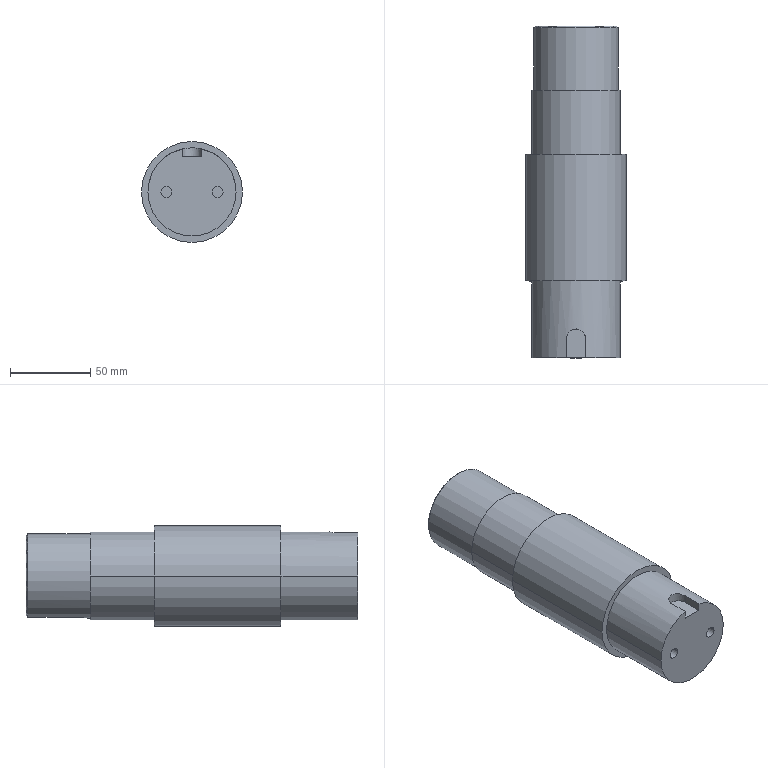Part | Creo | features CURVE 3, DATUM PLANE 3, CUT 2, ROUND 2, CHAMFER 1, COORDINATE SYSTEM 1, PROTRUSION 1 | 1 solid | 28 faces | box 63 x 207 x 63 mm | volume 538565 mm3 | cylinder 14 | plane 13 | cone 1 | commonest cylinder face diameters 6.8 x4 55 x4 12 x2 53 x2 63 x2
STEP:
#1=CARTESIAN_POINT('',(0.,0.,0.));
#2=DIRECTION('',(0.,0.,1.));
#3=DIRECTION('',(1.,0.,0.));
#4=AXIS2_PLACEMENT_3D('',#1,#2,#3);
#5=CARTESIAN_POINT('',(-6.,0.,26.837));
#6=VERTEX_POINT('',#5);
#7=CARTESIAN_POINT('',(-6.,0.,21.837));
#8=VERTEX_POINT('',#7);
#9=CARTESIAN_POINT('',(-6.,0.,26.837));
#10=DIRECTION('',(0.,0.,-1.));
#11=VECTOR('',#10,5.);
#12=LINE('',#9,#11);
#13=EDGE_CURVE('',#6,#8,#12,.T.);
#14=ORIENTED_EDGE('',*,*,#13,.T.);
#15=CARTESIAN_POINT('',(6.,0.,21.837));
#16=VERTEX_POINT('',#15);
#17=CARTESIAN_POINT('',(-6.,0.,21.837));
#18=DIRECTION('',(1.,0.,0.));
#19=VECTOR('',#18,12.);
#20=LINE('',#17,#19);
#21=EDGE_CURVE('',#8,#16,#20,.T.);
#22=ORIENTED_EDGE('',*,*,#21,.T.);
#23=CARTESIAN_POINT('',(6.,0.,26.837));
#24=VERTEX_POINT('',#23);
#25=CARTESIAN_POINT('',(6.,0.,21.837));
#26=DIRECTION('',(0.,0.,1.));
#27=VECTOR('',#26,5.);
#28=LINE('',#25,#27);
#29=EDGE_CURVE('',#16,#24,#28,.T.);
#30=ORIENTED_EDGE('',*,*,#29,.T.);
#31=CARTESIAN_POINT('',(27.5,0.,0.));
#32=VERTEX_POINT('',#31);
#33=CARTESIAN_POINT('',(0.,0.,0.));
#34=DIRECTION('',(0.,-1.,0.));
#35=DIRECTION('',(1.,0.,0.));
#36=AXIS2_PLACEMENT_3D('',#33,#34,#35);
#37=CIRCLE('',#36,27.5);
#38=EDGE_CURVE('',#32,#24,#37,.T.);
#39=ORIENTED_EDGE('',*,*,#38,.F.);
#40=CARTESIAN_POINT('',(-27.5,0.,0.));
#41=VERTEX_POINT('',#40);
#42=CARTESIAN_POINT('',(0.,0.,0.));
#43=DIRECTION('',(0.,1.,0.));
#44=DIRECTION('',(1.,0.,0.));
#45=AXIS2_PLACEMENT_3D('',#42,#43,#44);
#46=CIRCLE('',#45,27.5);
#47=EDGE_CURVE('',#32,#41,#46,.T.);
#48=ORIENTED_EDGE('',*,*,#47,.T.);
#49=CARTESIAN_POINT('',(0.,0.,0.));
#50=DIRECTION('',(0.,-1.,0.));
#51=DIRECTION('',(-0.2182,0.,0.9759));
#52=AXIS2_PLACEMENT_3D('',#49,#50,#51);
#53=CIRCLE('',#52,27.5);
#54=EDGE_CURVE('',#6,#41,#53,.T.);
#55=ORIENTED_EDGE('',*,*,#54,.F.);
#56=EDGE_LOOP('',(#14,#22,#30,#39,#48,#55));
#57=FACE_OUTER_BOUND('',#56,.F.);
#58=CARTESIAN_POINT('',(19.4,0.,0.));
#59=VERTEX_POINT('',#58);
#60=CARTESIAN_POINT('',(12.6,0.,0.));
#61=VERTEX_POINT('',#60);
#62=CARTESIAN_POINT('',(16.,0.,0.));
#63=DIRECTION('',(0.,-1.,0.));
#64=DIRECTION('',(1.,0.,0.));
#65=AXIS2_PLACEMENT_3D('',#62,#63,#64);
#66=CIRCLE('',#65,3.4);
#67=EDGE_CURVE('',#59,#61,#66,.T.);
#68=ORIENTED_EDGE('',*,*,#67,.T.);
#69=CARTESIAN_POINT('',(16.,0.,0.));
#70=DIRECTION('',(0.,-1.,0.));
#71=DIRECTION('',(-1.,0.,0.));
#72=AXIS2_PLACEMENT_3D('',#69,#70,#71);
#73=CIRCLE('',#72,3.4);
#74=EDGE_CURVE('',#61,#59,#73,.T.);
#75=ORIENTED_EDGE('',*,*,#74,.T.);
#76=EDGE_LOOP('',(#68,#75));
#77=FACE_BOUND('',#76,.F.);
#78=CARTESIAN_POINT('',(-12.6,0.,0.));
#79=VERTEX_POINT('',#78);
#80=CARTESIAN_POINT('',(-19.4,0.,0.));
#81=VERTEX_POINT('',#80);
#82=CARTESIAN_POINT('',(-16.,0.,0.));
#83=DIRECTION('',(0.,-1.,0.));
#84=DIRECTION('',(1.,0.,0.));
#85=AXIS2_PLACEMENT_3D('',#82,#83,#84);
#86=CIRCLE('',#85,3.4);
#87=EDGE_CURVE('',#79,#81,#86,.T.);
#88=ORIENTED_EDGE('',*,*,#87,.T.);
#89=CARTESIAN_POINT('',(-16.,0.,0.));
#90=DIRECTION('',(0.,-1.,0.));
#91=DIRECTION('',(-1.,0.,0.));
#92=AXIS2_PLACEMENT_3D('',#89,#90,#91);
#93=CIRCLE('',#92,3.4);
#94=EDGE_CURVE('',#81,#79,#93,.T.);
#95=ORIENTED_EDGE('',*,*,#94,.T.);
#96=EDGE_LOOP('',(#88,#95));
#97=FACE_BOUND('',#96,.F.);
#98=CARTESIAN_POINT('',(0.,0.,0.));
#99=DIRECTION('',(0.,1.,0.));
#100=DIRECTION('',(1.,0.,0.));
#101=AXIS2_PLACEMENT_3D('',#98,#99,#100);
#102=PLANE('',#101);
#103=ADVANCED_FACE('',(#57,#77,#97),#102,.F.);
#104=CARTESIAN_POINT('',(-6.,12.,21.837));
#105=VERTEX_POINT('',#104);
#106=CARTESIAN_POINT('',(-6.,12.,26.837));
#107=VERTEX_POINT('',#106);
#108=CARTESIAN_POINT('',(-6.,12.,21.837));
#109=DIRECTION('',(0.,0.,1.));
#110=VECTOR('',#109,5.);
#111=LINE('',#108,#110);
#112=EDGE_CURVE('',#105,#107,#111,.T.);
#113=ORIENTED_EDGE('',*,*,#112,.F.);
#114=CARTESIAN_POINT('',(-6.,0.,21.837));
#115=DIRECTION('',(0.,1.,0.));
#116=VECTOR('',#115,12.);
#117=LINE('',#114,#116);
#118=EDGE_CURVE('',#8,#105,#117,.T.);
#119=ORIENTED_EDGE('',*,*,#118,.F.);
#120=ORIENTED_EDGE('',*,*,#13,.F.);
#121=CARTESIAN_POINT('',(-6.,0.,26.837));
#122=DIRECTION('',(0.,1.,0.));
#123=VECTOR('',#122,12.);
#124=LINE('',#121,#123);
#125=EDGE_CURVE('',#6,#107,#124,.T.);
#126=ORIENTED_EDGE('',*,*,#125,.T.);
#127=EDGE_LOOP('',(#113,#119,#120,#126));
#128=FACE_OUTER_BOUND('',#127,.F.);
#129=CARTESIAN_POINT('',(-6.,0.,26.837));
#130=DIRECTION('',(-1.,0.,0.));
#131=DIRECTION('',(0.,0.,-1.));
#132=AXIS2_PLACEMENT_3D('',#129,#130,#131);
#133=PLANE('',#132);
#134=ADVANCED_FACE('',(#128),#133,.F.);
#135=CARTESIAN_POINT('',(6.,12.,26.837));
#136=VERTEX_POINT('',#135);
#137=CARTESIAN_POINT('',(6.,12.,21.837));
#138=VERTEX_POINT('',#137);
#139=CARTESIAN_POINT('',(6.,12.,26.837));
#140=DIRECTION('',(0.,0.,-1.));
#141=VECTOR('',#140,5.);
#142=LINE('',#139,#141);
#143=EDGE_CURVE('',#136,#138,#142,.T.);
#144=ORIENTED_EDGE('',*,*,#143,.T.);
#145=CARTESIAN_POINT('',(0.,12.,21.837));
#146=DIRECTION('',(0.,0.,-1.));
#147=DIRECTION('',(-1.,0.,0.));
#148=AXIS2_PLACEMENT_3D('',#145,#146,#147);
#149=CIRCLE('',#148,6.);
#150=EDGE_CURVE('',#105,#138,#149,.T.);
#151=ORIENTED_EDGE('',*,*,#150,.F.);
#152=ORIENTED_EDGE('',*,*,#112,.T.);
#153=CARTESIAN_POINT('',(6.,12.,26.837));
#154=CARTESIAN_POINT('',(6.,12.529,26.837));
#155=CARTESIAN_POINT('',(5.865,13.55,26.868));
#156=CARTESIAN_POINT('',(5.265,15.022,26.995));
#157=CARTESIAN_POINT('',(4.293,16.292,27.171));
#158=CARTESIAN_POINT('',(3.022,17.264,27.345));
#159=CARTESIAN_POINT('',(1.556,17.865,27.47));
#160=CARTESIAN_POINT('',(0.,18.067,27.515));
#161=CARTESIAN_POINT('',(-1.556,17.865,27.47));
#162=CARTESIAN_POINT('',(-3.022,17.264,27.345));
#163=CARTESIAN_POINT('',(-4.293,16.292,27.171));
#164=CARTESIAN_POINT('',(-5.265,15.022,26.995));
#165=CARTESIAN_POINT('',(-5.865,13.55,26.868));
#166=CARTESIAN_POINT('',(-6.,12.529,26.837));
#167=CARTESIAN_POINT('',(-6.,12.,26.837));
#168=B_SPLINE_CURVE_WITH_KNOTS('',3,(#153,#154,#155,#156,#157,#158,#159,#160,#161,#162,#163,#164,#165,#166,#167),.UNSPECIFIED.,.F.,.F.,(4,1,1,1,1,1,1,1,1,1,1,1,4),(0.,0.08333,0.1667,0.25,0.3333,0.4167,0.5,0.5833,0.6667,0.75,0.8333,0.9167,1.),.UNSPECIFIED.);
#169=EDGE_CURVE('',#136,#107,#168,.T.);
#170=ORIENTED_EDGE('',*,*,#169,.F.);
#171=EDGE_LOOP('',(#144,#151,#152,#170));
#172=FACE_OUTER_BOUND('',#171,.F.);
#173=CARTESIAN_POINT('',(0.,12.,113.768));
#174=DIRECTION('',(0.,0.,-1.));
#175=DIRECTION('',(0.,1.,0.));
#176=AXIS2_PLACEMENT_3D('',#173,#174,#175);
#177=CYLINDRICAL_SURFACE('',#176,6.);
#178=ADVANCED_FACE('',(#172),#177,.F.);
#179=ORIENTED_EDGE('',*,*,#143,.F.);
#180=CARTESIAN_POINT('',(6.,0.,26.837));
#181=DIRECTION('',(0.,1.,0.));
#182=VECTOR('',#181,12.);
#183=LINE('',#180,#182);
#184=EDGE_CURVE('',#24,#136,#183,.T.);
#185=ORIENTED_EDGE('',*,*,#184,.F.);
#186=ORIENTED_EDGE('',*,*,#29,.F.);
#187=CARTESIAN_POINT('',(6.,0.,21.837));
#188=DIRECTION('',(0.,1.,0.));
#189=VECTOR('',#188,12.);
#190=LINE('',#187,#189);
#191=EDGE_CURVE('',#16,#138,#190,.T.);
#192=ORIENTED_EDGE('',*,*,#191,.T.);
#193=EDGE_LOOP('',(#179,#185,#186,#192));
#194=FACE_OUTER_BOUND('',#193,.F.);
#195=CARTESIAN_POINT('',(6.,0.,21.837));
#196=DIRECTION('',(1.,0.,0.));
#197=DIRECTION('',(0.,0.,1.));
#198=AXIS2_PLACEMENT_3D('',#195,#196,#197);
#199=PLANE('',#198);
#200=ADVANCED_FACE('',(#194),#199,.F.);
#201=ORIENTED_EDGE('',*,*,#184,.T.);
#202=ORIENTED_EDGE('',*,*,#169,.T.);
#203=ORIENTED_EDGE('',*,*,#125,.F.);
#204=ORIENTED_EDGE('',*,*,#54,.T.);
#205=CARTESIAN_POINT('',(-27.5,48.,0.));
#206=VERTEX_POINT('',#205);
#207=CARTESIAN_POINT('',(-27.5,0.,0.));
#208=DIRECTION('',(0.,1.,0.));
#209=VECTOR('',#208,48.);
#210=LINE('',#207,#209);
#211=EDGE_CURVE('',#41,#206,#210,.T.);
#212=ORIENTED_EDGE('',*,*,#211,.T.);
#213=CARTESIAN_POINT('',(27.5,48.,0.));
#214=VERTEX_POINT('',#213);
#215=CARTESIAN_POINT('',(0.,48.,0.));
#216=DIRECTION('',(0.,-1.,0.));
#217=DIRECTION('',(1.,0.,0.));
#218=AXIS2_PLACEMENT_3D('',#215,#216,#217);
#219=CIRCLE('',#218,27.5);
#220=EDGE_CURVE('',#214,#206,#219,.T.);
#221=ORIENTED_EDGE('',*,*,#220,.F.);
#222=CARTESIAN_POINT('',(27.5,0.,0.));
#223=DIRECTION('',(0.,1.,0.));
#224=VECTOR('',#223,48.);
#225=LINE('',#222,#224);
#226=EDGE_CURVE('',#32,#214,#225,.T.);
#227=ORIENTED_EDGE('',*,*,#226,.F.);
#228=ORIENTED_EDGE('',*,*,#38,.T.);
#229=EDGE_LOOP('',(#201,#202,#203,#204,#212,#221,#227,#228));
#230=FACE_OUTER_BOUND('',#229,.F.);
#231=CARTESIAN_POINT('',(0.,0.,0.));
#232=DIRECTION('',(0.,1.,0.));
#233=DIRECTION('',(1.,0.,0.));
#234=AXIS2_PLACEMENT_3D('',#231,#232,#233);
#235=CYLINDRICAL_SURFACE('',#234,27.5);
#236=ADVANCED_FACE('',(#230),#235,.T.);
#237=ORIENTED_EDGE('',*,*,#226,.T.);
#238=CARTESIAN_POINT('',(0.,48.,0.));
#239=DIRECTION('',(0.,1.,0.));
#240=DIRECTION('',(1.,0.,0.));
#241=AXIS2_PLACEMENT_3D('',#238,#239,#240);
#242=CIRCLE('',#241,27.5);
#243=EDGE_CURVE('',#214,#206,#242,.T.);
#244=ORIENTED_EDGE('',*,*,#243,.T.);
#245=ORIENTED_EDGE('',*,*,#211,.F.);
#246=ORIENTED_EDGE('',*,*,#47,.F.);
#247=EDGE_LOOP('',(#237,#244,#245,#246));
#248=FACE_OUTER_BOUND('',#247,.F.);
#249=CARTESIAN_POINT('',(0.,0.,0.));
#250=DIRECTION('',(0.,1.,0.));
#251=DIRECTION('',(1.,0.,0.));
#252=AXIS2_PLACEMENT_3D('',#249,#250,#251);
#253=CYLINDRICAL_SURFACE('',#252,27.5);
#254=ADVANCED_FACE('',(#248),#253,.T.);
#255=CARTESIAN_POINT('',(31.5,48.,0.));
#256=VERTEX_POINT('',#255);
#257=CARTESIAN_POINT('',(-31.5,48.,0.));
#258=VERTEX_POINT('',#257);
#259=CARTESIAN_POINT('',(0.,48.,0.));
#260=DIRECTION('',(0.,1.,0.));
#261=DIRECTION('',(1.,0.,0.));
#262=AXIS2_PLACEMENT_3D('',#259,#260,#261);
#263=CIRCLE('',#262,31.5);
#264=EDGE_CURVE('',#256,#258,#263,.T.);
#265=ORIENTED_EDGE('',*,*,#264,.T.);
#266=CARTESIAN_POINT('',(0.,48.,0.));
#267=DIRECTION('',(0.,-1.,0.));
#268=DIRECTION('',(1.,0.,0.));
#269=AXIS2_PLACEMENT_3D('',#266,#267,#268);
#270=CIRCLE('',#269,31.5);
#271=EDGE_CURVE('',#256,#258,#270,.T.);
#272=ORIENTED_EDGE('',*,*,#271,.F.);
#273=EDGE_LOOP('',(#265,#272));
#274=FACE_OUTER_BOUND('',#273,.F.);
#275=ORIENTED_EDGE('',*,*,#220,.T.);
#276=ORIENTED_EDGE('',*,*,#243,.F.);
#277=EDGE_LOOP('',(#275,#276));
#278=FACE_BOUND('',#277,.F.);
#279=CARTESIAN_POINT('',(0.,48.,0.));
#280=DIRECTION('',(0.,1.,0.));
#281=DIRECTION('',(1.,0.,0.));
#282=AXIS2_PLACEMENT_3D('',#279,#280,#281);
#283=PLANE('',#282);
#284=ADVANCED_FACE('',(#274,#278),#283,.F.);
#285=CARTESIAN_POINT('',(31.5,127.,0.));
#286=VERTEX_POINT('',#285);
#287=CARTESIAN_POINT('',(31.5,48.,0.));
#288=DIRECTION('',(0.,1.,0.));
#289=VECTOR('',#288,79.);
#290=LINE('',#287,#289);
#291=EDGE_CURVE('',#256,#286,#290,.T.);
#292=ORIENTED_EDGE('',*,*,#291,.T.);
#293=CARTESIAN_POINT('',(-31.5,127.,0.));
#294=VERTEX_POINT('',#293);
#295=CARTESIAN_POINT('',(0.,127.,0.));
#296=DIRECTION('',(0.,1.,0.));
#297=DIRECTION('',(1.,0.,0.));
#298=AXIS2_PLACEMENT_3D('',#295,#296,#297);
#299=CIRCLE('',#298,31.5);
#300=EDGE_CURVE('',#286,#294,#299,.T.);
#301=ORIENTED_EDGE('',*,*,#300,.T.);
#302=CARTESIAN_POINT('',(-31.5,48.,0.));
#303=DIRECTION('',(0.,1.,0.));
#304=VECTOR('',#303,79.);
#305=LINE('',#302,#304);
#306=EDGE_CURVE('',#258,#294,#305,.T.);
#307=ORIENTED_EDGE('',*,*,#306,.F.);
#308=ORIENTED_EDGE('',*,*,#264,.F.);
#309=EDGE_LOOP('',(#292,#301,#307,#308));
#310=FACE_OUTER_BOUND('',#309,.F.);
#311=CARTESIAN_POINT('',(0.,0.,0.));
#312=DIRECTION('',(0.,1.,0.));
#313=DIRECTION('',(1.,0.,0.));
#314=AXIS2_PLACEMENT_3D('',#311,#312,#313);
#315=CYLINDRICAL_SURFACE('',#314,31.5);
#316=ADVANCED_FACE('',(#310),#315,.T.);
#317=ORIENTED_EDGE('',*,*,#291,.F.);
#318=ORIENTED_EDGE('',*,*,#271,.T.);
#319=ORIENTED_EDGE('',*,*,#306,.T.);
#320=CARTESIAN_POINT('',(0.,127.,0.));
#321=DIRECTION('',(0.,-1.,0.));
#322=DIRECTION('',(1.,0.,0.));
#323=AXIS2_PLACEMENT_3D('',#320,#321,#322);
#324=CIRCLE('',#323,31.5);
#325=EDGE_CURVE('',#286,#294,#324,.T.);
#326=ORIENTED_EDGE('',*,*,#325,.F.);
#327=EDGE_LOOP('',(#317,#318,#319,#326));
#328=FACE_OUTER_BOUND('',#327,.F.);
#329=CARTESIAN_POINT('',(0.,0.,0.));
#330=DIRECTION('',(0.,1.,0.));
#331=DIRECTION('',(1.,0.,0.));
#332=AXIS2_PLACEMENT_3D('',#329,#330,#331);
#333=CYLINDRICAL_SURFACE('',#332,31.5);
#334=ADVANCED_FACE('',(#328),#333,.T.);
#335=ORIENTED_EDGE('',*,*,#325,.T.);
#336=ORIENTED_EDGE('',*,*,#300,.F.);
#337=EDGE_LOOP('',(#335,#336));
#338=FACE_OUTER_BOUND('',#337,.F.);
#339=CARTESIAN_POINT('',(27.5,127.,0.));
#340=VERTEX_POINT('',#339);
#341=CARTESIAN_POINT('',(-27.5,127.,0.));
#342=VERTEX_POINT('',#341);
#343=CARTESIAN_POINT('',(0.,127.,0.));
#344=DIRECTION('',(0.,1.,0.));
#345=DIRECTION('',(1.,0.,0.));
#346=AXIS2_PLACEMENT_3D('',#343,#344,#345);
#347=CIRCLE('',#346,27.5);
#348=EDGE_CURVE('',#340,#342,#347,.T.);
#349=ORIENTED_EDGE('',*,*,#348,.T.);
#350=CARTESIAN_POINT('',(0.,127.,0.));
#351=DIRECTION('',(0.,-1.,0.));
#352=DIRECTION('',(1.,0.,0.));
#353=AXIS2_PLACEMENT_3D('',#350,#351,#352);
#354=CIRCLE('',#353,27.5);
#355=EDGE_CURVE('',#340,#342,#354,.T.);
#356=ORIENTED_EDGE('',*,*,#355,.F.);
#357=EDGE_LOOP('',(#349,#356));
#358=FACE_BOUND('',#357,.F.);
#359=CARTESIAN_POINT('',(0.,127.,0.));
#360=DIRECTION('',(0.,1.,0.));
#361=DIRECTION('',(1.,0.,0.));
#362=AXIS2_PLACEMENT_3D('',#359,#360,#361);
#363=PLANE('',#362);
#364=ADVANCED_FACE('',(#338,#358),#363,.T.);
#365=CARTESIAN_POINT('',(27.5,167.,0.));
#366=VERTEX_POINT('',#365);
#367=CARTESIAN_POINT('',(27.5,127.,0.));
#368=DIRECTION('',(0.,1.,0.));
#369=VECTOR('',#368,40.);
#370=LINE('',#367,#369);
#371=EDGE_CURVE('',#340,#366,#370,.T.);
#372=ORIENTED_EDGE('',*,*,#371,.T.);
#373=CARTESIAN_POINT('',(-27.5,167.,0.));
#374=VERTEX_POINT('',#373);
#375=CARTESIAN_POINT('',(0.,167.,0.));
#376=DIRECTION('',(0.,1.,0.));
#377=DIRECTION('',(1.,0.,0.));
#378=AXIS2_PLACEMENT_3D('',#375,#376,#377);
#379=CIRCLE('',#378,27.5);
#380=EDGE_CURVE('',#366,#374,#379,.T.);
#381=ORIENTED_EDGE('',*,*,#380,.T.);
#382=CARTESIAN_POINT('',(-27.5,127.,0.));
#383=DIRECTION('',(0.,1.,0.));
#384=VECTOR('',#383,40.);
#385=LINE('',#382,#384);
#386=EDGE_CURVE('',#342,#374,#385,.T.);
#387=ORIENTED_EDGE('',*,*,#386,.F.);
#388=ORIENTED_EDGE('',*,*,#348,.F.);
#389=EDGE_LOOP('',(#372,#381,#387,#388));
#390=FACE_OUTER_BOUND('',#389,.F.);
#391=CARTESIAN_POINT('',(0.,0.,0.));
#392=DIRECTION('',(0.,1.,0.));
#393=DIRECTION('',(1.,0.,0.));
#394=AXIS2_PLACEMENT_3D('',#391,#392,#393);
#395=CYLINDRICAL_SURFACE('',#394,27.5);
#396=ADVANCED_FACE('',(#390),#395,.T.);
#397=ORIENTED_EDGE('',*,*,#371,.F.);
#398=ORIENTED_EDGE('',*,*,#355,.T.);
#399=ORIENTED_EDGE('',*,*,#386,.T.);
#400=CARTESIAN_POINT('',(0.,167.,0.));
#401=DIRECTION('',(0.,-1.,0.));
#402=DIRECTION('',(1.,0.,0.));
#403=AXIS2_PLACEMENT_3D('',#400,#401,#402);
#404=CIRCLE('',#403,27.5);
#405=EDGE_CURVE('',#366,#374,#404,.T.);
#406=ORIENTED_EDGE('',*,*,#405,.F.);
#407=EDGE_LOOP('',(#397,#398,#399,#406));
#408=FACE_OUTER_BOUND('',#407,.F.);
#409=CARTESIAN_POINT('',(0.,0.,0.));
#410=DIRECTION('',(0.,1.,0.));
#411=DIRECTION('',(1.,0.,0.));
#412=AXIS2_PLACEMENT_3D('',#409,#410,#411);
#413=CYLINDRICAL_SURFACE('',#412,27.5);
#414=ADVANCED_FACE('',(#408),#413,.T.);
#415=ORIENTED_EDGE('',*,*,#405,.T.);
#416=ORIENTED_EDGE('',*,*,#380,.F.);
#417=EDGE_LOOP('',(#415,#416));
#418=FACE_OUTER_BOUND('',#417,.F.);
#419=CARTESIAN_POINT('',(6.,167.,-25.812));
#420=VERTEX_POINT('',#419);
#421=CARTESIAN_POINT('',(0.,167.,-26.5));
#422=VERTEX_POINT('',#421);
#423=CARTESIAN_POINT('',(0.,167.,0.));
#424=DIRECTION('',(0.,-1.,0.));
#425=DIRECTION('',(0.2264,0.,-0.974));
#426=AXIS2_PLACEMENT_3D('',#423,#424,#425);
#427=CIRCLE('',#426,26.5);
#428=EDGE_CURVE('',#420,#422,#427,.T.);
#429=ORIENTED_EDGE('',*,*,#428,.F.);
#430=CARTESIAN_POINT('',(0.,167.,0.));
#431=DIRECTION('',(0.,-1.,0.));
#432=DIRECTION('',(0.,0.,-1.));
#433=AXIS2_PLACEMENT_3D('',#430,#431,#432);
#434=CIRCLE('',#433,26.5);
#435=EDGE_CURVE('',#422,#420,#434,.T.);
#436=ORIENTED_EDGE('',*,*,#435,.F.);
#437=EDGE_LOOP('',(#429,#436));
#438=FACE_BOUND('',#437,.F.);
#439=CARTESIAN_POINT('',(0.,167.,0.));
#440=DIRECTION('',(0.,1.,0.));
#441=DIRECTION('',(1.,0.,0.));
#442=AXIS2_PLACEMENT_3D('',#439,#440,#441);
#443=PLANE('',#442);
#444=ADVANCED_FACE('',(#418,#438),#443,.T.);
#445=CARTESIAN_POINT('',(6.,206.,-25.812));
#446=VERTEX_POINT('',#445);
#447=CARTESIAN_POINT('',(-6.,206.,-25.812));
#448=VERTEX_POINT('',#447);
#449=CARTESIAN_POINT('',(0.0001348,206.,-0.000703));
#450=DIRECTION('',(0.,-1.,0.));
#451=DIRECTION('',(0.2264,0.,-0.974));
#452=AXIS2_PLACEMENT_3D('',#449,#450,#451);
#453=CIRCLE('',#452,26.5);
#454=EDGE_CURVE('',#446,#448,#453,.T.);
#455=ORIENTED_EDGE('',*,*,#454,.F.);
#456=CARTESIAN_POINT('',(6.,173.,-25.812));
#457=VERTEX_POINT('',#456);
#458=CARTESIAN_POINT('',(6.,173.,-25.812));
#459=DIRECTION('',(0.000000811,1.,-0.000003487));
#460=VECTOR('',#459,33.);
#461=LINE('',#458,#460);
#462=EDGE_CURVE('',#457,#446,#461,.T.);
#463=ORIENTED_EDGE('',*,*,#462,.F.);
#464=CARTESIAN_POINT('',(6.,167.,-25.812));
#465=DIRECTION('',(0.,1.,0.));
#466=VECTOR('',#465,6.);
#467=LINE('',#464,#466);
#468=EDGE_CURVE('',#420,#457,#467,.T.);
#469=ORIENTED_EDGE('',*,*,#468,.F.);
#470=ORIENTED_EDGE('',*,*,#428,.T.);
#471=CARTESIAN_POINT('',(-6.,173.,-25.812));
#472=VERTEX_POINT('',#471);
#473=CARTESIAN_POINT('',(-6.,173.,-25.812));
#474=CARTESIAN_POINT('',(-6.,172.482,-25.812));
#475=CARTESIAN_POINT('',(-5.866,171.442,-25.844));
#476=CARTESIAN_POINT('',(-5.26,169.971,-25.977));
#477=CARTESIAN_POINT('',(-4.292,168.709,-26.158));
#478=CARTESIAN_POINT('',(-3.029,167.74,-26.339));
#479=CARTESIAN_POINT('',(-1.558,167.135,-26.469));
#480=CARTESIAN_POINT('',(-0.5181,167.,-26.5));
#481=CARTESIAN_POINT('',(0.,167.,-26.5));
#482=B_SPLINE_CURVE_WITH_KNOTS('',3,(#473,#474,#475,#476,#477,#478,#479,#480,#481),.UNSPECIFIED.,.F.,.F.,(4,1,1,1,1,1,4),(0.,0.1667,0.3333,0.5,0.6667,0.8333,1.),.UNSPECIFIED.);
#483=EDGE_CURVE('',#472,#422,#482,.T.);
#484=ORIENTED_EDGE('',*,*,#483,.F.);
#485=CARTESIAN_POINT('',(-6.,173.,-25.812));
#486=DIRECTION('',(0.000000895,1.,-0.000003491));
#487=VECTOR('',#486,33.);
#488=LINE('',#485,#487);
#489=EDGE_CURVE('',#472,#448,#488,.T.);
#490=ORIENTED_EDGE('',*,*,#489,.T.);
#491=EDGE_LOOP('',(#455,#463,#469,#470,#484,#490));
#492=FACE_OUTER_BOUND('',#491,.F.);
#493=CARTESIAN_POINT('',(0.,0.,0.));
#494=DIRECTION('',(0.,1.,0.));
#495=DIRECTION('',(1.,0.,0.));
#496=AXIS2_PLACEMENT_3D('',#493,#494,#495);
#497=CYLINDRICAL_SURFACE('',#496,26.5);
#498=ADVANCED_FACE('',(#492),#497,.T.);
#499=ORIENTED_EDGE('',*,*,#454,.T.);
#500=CARTESIAN_POINT('',(-6.,207.,-24.784));
#501=VERTEX_POINT('',#500);
#502=CARTESIAN_POINT('',(-6.,206.169,-25.638));
#503=CARTESIAN_POINT('',(-6.,206.505,-25.294));
#504=CARTESIAN_POINT('',(-6.,206.836,-24.953));
#505=B_SPLINE_CURVE_WITH_KNOTS('',3,(#447,#502,#503,#504,#500),.UNSPECIFIED.,.F.,.F.,(4,1,4),(0.,0.5,1.),.UNSPECIFIED.);
#506=EDGE_CURVE('',#448,#501,#505,.T.);
#507=ORIENTED_EDGE('',*,*,#506,.T.);
#508=CARTESIAN_POINT('',(6.,207.,-24.784));
#509=VERTEX_POINT('',#508);
#510=CARTESIAN_POINT('',(0.0001348,207.,-0.000703));
#511=DIRECTION('',(0.,1.,0.));
#512=DIRECTION('',(-0.2353,0.,-0.9719));
#513=AXIS2_PLACEMENT_3D('',#510,#511,#512);
#514=CIRCLE('',#513,25.5);
#515=EDGE_CURVE('',#501,#509,#514,.T.);
#516=ORIENTED_EDGE('',*,*,#515,.T.);
#517=CARTESIAN_POINT('',(6.,206.836,-24.953));
#518=CARTESIAN_POINT('',(6.,206.506,-25.294));
#519=CARTESIAN_POINT('',(6.,206.169,-25.638));
#520=B_SPLINE_CURVE_WITH_KNOTS('',3,(#508,#517,#518,#519,#445),.UNSPECIFIED.,.F.,.F.,(4,1,4),(0.,0.5,1.),.UNSPECIFIED.);
#521=EDGE_CURVE('',#509,#446,#520,.T.);
#522=ORIENTED_EDGE('',*,*,#521,.T.);
#523=EDGE_LOOP('',(#499,#507,#516,#522));
#524=FACE_OUTER_BOUND('',#523,.F.);
#525=CARTESIAN_POINT('',(0.0001348,206.5,-0.000703));
#526=DIRECTION('',(0.,-1.,0.));
#527=DIRECTION('',(0.,0.,-1.));
#528=AXIS2_PLACEMENT_3D('',#525,#526,#527);
#529=CONICAL_SURFACE('',#528,26.,45.001);
#530=ADVANCED_FACE('',(#524),#529,.T.);
#531=ORIENTED_EDGE('',*,*,#506,.F.);
#532=ORIENTED_EDGE('',*,*,#489,.F.);
#533=CARTESIAN_POINT('',(-6.,173.,-20.812));
#534=VERTEX_POINT('',#533);
#535=CARTESIAN_POINT('',(-6.,173.,-20.812));
#536=DIRECTION('',(0.,0.,-1.));
#537=VECTOR('',#536,5.);
#538=LINE('',#535,#537);
#539=EDGE_CURVE('',#534,#472,#538,.T.);
#540=ORIENTED_EDGE('',*,*,#539,.F.);
#541=CARTESIAN_POINT('',(-6.,207.,-20.812));
#542=VERTEX_POINT('',#541);
#543=CARTESIAN_POINT('',(-6.,207.,-20.812));
#544=DIRECTION('',(0.,-1.,0.));
#545=VECTOR('',#544,34.);
#546=LINE('',#543,#545);
#547=EDGE_CURVE('',#542,#534,#546,.T.);
#548=ORIENTED_EDGE('',*,*,#547,.F.);
#549=CARTESIAN_POINT('',(-6.,207.,-24.784));
#550=DIRECTION('',(-0.00000746,-0.00002661,1.));
#551=VECTOR('',#550,3.972);
#552=LINE('',#549,#551);
#553=EDGE_CURVE('',#501,#542,#552,.T.);
#554=ORIENTED_EDGE('',*,*,#553,.F.);
#555=EDGE_LOOP('',(#531,#532,#540,#548,#554));
#556=FACE_OUTER_BOUND('',#555,.F.);
#557=CARTESIAN_POINT('',(-6.,207.,-25.812));
#558=DIRECTION('',(-1.,0.,0.));
#559=DIRECTION('',(0.,0.,1.));
#560=AXIS2_PLACEMENT_3D('',#557,#558,#559);
#561=PLANE('',#560);
#562=ADVANCED_FACE('',(#556),#561,.F.);
#563=CARTESIAN_POINT('',(6.,173.,-20.812));
#564=VERTEX_POINT('',#563);
#565=CARTESIAN_POINT('',(6.,173.,-25.812));
#566=DIRECTION('',(0.,0.,1.));
#567=VECTOR('',#566,5.);
#568=LINE('',#565,#567);
#569=EDGE_CURVE('',#457,#564,#568,.T.);
#570=ORIENTED_EDGE('',*,*,#569,.T.);
#571=CARTESIAN_POINT('',(0.,173.,-20.812));
#572=DIRECTION('',(0.,0.,1.));
#573=DIRECTION('',(-1.,0.,0.));
#574=AXIS2_PLACEMENT_3D('',#571,#572,#573);
#575=CIRCLE('',#574,6.);
#576=EDGE_CURVE('',#534,#564,#575,.T.);
#577=ORIENTED_EDGE('',*,*,#576,.F.);
#578=ORIENTED_EDGE('',*,*,#539,.T.);
#579=ORIENTED_EDGE('',*,*,#483,.T.);
#580=CARTESIAN_POINT('',(0.,167.,-26.5));
#581=CARTESIAN_POINT('',(0.5181,167.,-26.5));
#582=CARTESIAN_POINT('',(1.558,167.135,-26.469));
#583=CARTESIAN_POINT('',(3.029,167.74,-26.339));
#584=CARTESIAN_POINT('',(4.292,168.709,-26.158));
#585=CARTESIAN_POINT('',(5.26,169.971,-25.977));
#586=CARTESIAN_POINT('',(5.866,171.442,-25.844));
#587=CARTESIAN_POINT('',(6.,172.482,-25.812));
#588=CARTESIAN_POINT('',(6.,173.,-25.812));
#589=B_SPLINE_CURVE_WITH_KNOTS('',3,(#580,#581,#582,#583,#584,#585,#586,#587,#588),.UNSPECIFIED.,.F.,.F.,(4,1,1,1,1,1,4),(0.,0.1667,0.3333,0.5,0.6667,0.8333,1.),.UNSPECIFIED.);
#590=EDGE_CURVE('',#422,#457,#589,.T.);
#591=ORIENTED_EDGE('',*,*,#590,.T.);
#592=EDGE_LOOP('',(#570,#577,#578,#579,#591));
#593=FACE_OUTER_BOUND('',#592,.F.);
#594=CARTESIAN_POINT('',(0.,173.,-113.768));
#595=DIRECTION('',(0.,0.,1.));
#596=DIRECTION('',(0.,-1.,0.));
#597=AXIS2_PLACEMENT_3D('',#594,#595,#596);
#598=CYLINDRICAL_SURFACE('',#597,6.);
#599=ADVANCED_FACE('',(#593),#598,.F.);
#600=ORIENTED_EDGE('',*,*,#521,.F.);
#601=CARTESIAN_POINT('',(6.,207.,-20.812));
#602=VERTEX_POINT('',#601);
#603=CARTESIAN_POINT('',(6.,207.,-20.812));
#604=DIRECTION('',(0.000006729,0.0000286,-1.));
#605=VECTOR('',#604,3.972);
#606=LINE('',#603,#605);
#607=EDGE_CURVE('',#602,#509,#606,.T.);
#608=ORIENTED_EDGE('',*,*,#607,.F.);
#609=CARTESIAN_POINT('',(6.,207.,-20.812));
#610=DIRECTION('',(0.,-1.,0.));
#611=VECTOR('',#610,34.);
#612=LINE('',#609,#611);
#613=EDGE_CURVE('',#602,#564,#612,.T.);
#614=ORIENTED_EDGE('',*,*,#613,.T.);
#615=ORIENTED_EDGE('',*,*,#569,.F.);
#616=ORIENTED_EDGE('',*,*,#462,.T.);
#617=EDGE_LOOP('',(#600,#608,#614,#615,#616));
#618=FACE_OUTER_BOUND('',#617,.F.);
#619=CARTESIAN_POINT('',(6.,207.,-20.812));
#620=DIRECTION('',(1.,0.,0.));
#621=DIRECTION('',(0.,0.,-1.));
#622=AXIS2_PLACEMENT_3D('',#619,#620,#621);
#623=PLANE('',#622);
#624=ADVANCED_FACE('',(#618),#623,.F.);
#625=ORIENTED_EDGE('',*,*,#515,.F.);
#626=ORIENTED_EDGE('',*,*,#553,.T.);
#627=CARTESIAN_POINT('',(-6.,207.,-20.812));
#628=DIRECTION('',(1.,0.,0.));
#629=VECTOR('',#628,12.);
#630=LINE('',#627,#629);
#631=EDGE_CURVE('',#542,#602,#630,.T.);
#632=ORIENTED_EDGE('',*,*,#631,.T.);
#633=ORIENTED_EDGE('',*,*,#607,.T.);
#634=EDGE_LOOP('',(#625,#626,#632,#633));
#635=FACE_OUTER_BOUND('',#634,.F.);
#636=CARTESIAN_POINT('',(0.,207.,0.));
#637=DIRECTION('',(0.,1.,0.));
#638=DIRECTION('',(1.,0.,0.));
#639=AXIS2_PLACEMENT_3D('',#636,#637,#638);
#640=PLANE('',#639);
#641=ADVANCED_FACE('',(#635),#640,.T.);
#642=ORIENTED_EDGE('',*,*,#576,.T.);
#643=ORIENTED_EDGE('',*,*,#613,.F.);
#644=ORIENTED_EDGE('',*,*,#631,.F.);
#645=ORIENTED_EDGE('',*,*,#547,.T.);
#646=EDGE_LOOP('',(#642,#643,#644,#645));
#647=FACE_OUTER_BOUND('',#646,.F.);
#648=CARTESIAN_POINT('',(-6.,207.,-20.812));
#649=DIRECTION('',(0.,0.,1.));
#650=DIRECTION('',(1.,0.,0.));
#651=AXIS2_PLACEMENT_3D('',#648,#649,#650);
#652=PLANE('',#651);
#653=ADVANCED_FACE('',(#647),#652,.F.);
#654=ORIENTED_EDGE('',*,*,#435,.T.);
#655=ORIENTED_EDGE('',*,*,#468,.T.);
#656=ORIENTED_EDGE('',*,*,#590,.F.);
#657=EDGE_LOOP('',(#654,#655,#656));
#658=FACE_OUTER_BOUND('',#657,.F.);
#659=CARTESIAN_POINT('',(0.,0.,0.));
#660=DIRECTION('',(0.,1.,0.));
#661=DIRECTION('',(1.,0.,0.));
#662=AXIS2_PLACEMENT_3D('',#659,#660,#661);
#663=CYLINDRICAL_SURFACE('',#662,26.5);
#664=ADVANCED_FACE('',(#658),#663,.T.);
#665=ORIENTED_EDGE('',*,*,#150,.T.);
#666=ORIENTED_EDGE('',*,*,#191,.F.);
#667=ORIENTED_EDGE('',*,*,#21,.F.);
#668=ORIENTED_EDGE('',*,*,#118,.T.);
#669=EDGE_LOOP('',(#665,#666,#667,#668));
#670=FACE_OUTER_BOUND('',#669,.F.);
#671=CARTESIAN_POINT('',(-6.,0.,21.837));
#672=DIRECTION('',(0.,0.,-1.));
#673=DIRECTION('',(1.,0.,0.));
#674=AXIS2_PLACEMENT_3D('',#671,#672,#673);
#675=PLANE('',#674);
#676=ADVANCED_FACE('',(#670),#675,.F.);
#677=ORIENTED_EDGE('',*,*,#67,.F.);
#678=CARTESIAN_POINT('',(19.4,18.,0.));
#679=VERTEX_POINT('',#678);
#680=CARTESIAN_POINT('',(19.4,0.,0.));
#681=DIRECTION('',(0.,1.,0.));
#682=VECTOR('',#681,18.);
#683=LINE('',#680,#682);
#684=EDGE_CURVE('',#59,#679,#683,.T.);
#685=ORIENTED_EDGE('',*,*,#684,.T.);
#686=CARTESIAN_POINT('',(12.6,18.,0.));
#687=VERTEX_POINT('',#686);
#688=CARTESIAN_POINT('',(16.,18.,0.));
#689=DIRECTION('',(0.,-1.,0.));
#690=DIRECTION('',(1.,0.,0.));
#691=AXIS2_PLACEMENT_3D('',#688,#689,#690);
#692=CIRCLE('',#691,3.4);
#693=EDGE_CURVE('',#679,#687,#692,.T.);
#694=ORIENTED_EDGE('',*,*,#693,.T.);
#695=CARTESIAN_POINT('',(12.6,0.,0.));
#696=DIRECTION('',(0.,1.,0.));
#697=VECTOR('',#696,18.);
#698=LINE('',#695,#697);
#699=EDGE_CURVE('',#61,#687,#698,.T.);
#700=ORIENTED_EDGE('',*,*,#699,.F.);
#701=EDGE_LOOP('',(#677,#685,#694,#700));
#702=FACE_OUTER_BOUND('',#701,.F.);
#703=CARTESIAN_POINT('',(16.,0.,0.));
#704=DIRECTION('',(0.,-1.,0.));
#705=DIRECTION('',(1.,0.,0.));
#706=AXIS2_PLACEMENT_3D('',#703,#704,#705);
#707=CYLINDRICAL_SURFACE('',#706,3.4);
#708=ADVANCED_FACE('',(#702),#707,.F.);
#709=ORIENTED_EDGE('',*,*,#74,.F.);
#710=ORIENTED_EDGE('',*,*,#699,.T.);
#711=CARTESIAN_POINT('',(16.,18.,0.));
#712=DIRECTION('',(0.,-1.,0.));
#713=DIRECTION('',(-1.,0.,0.));
#714=AXIS2_PLACEMENT_3D('',#711,#712,#713);
#715=CIRCLE('',#714,3.4);
#716=EDGE_CURVE('',#687,#679,#715,.T.);
#717=ORIENTED_EDGE('',*,*,#716,.T.);
#718=ORIENTED_EDGE('',*,*,#684,.F.);
#719=EDGE_LOOP('',(#709,#710,#717,#718));
#720=FACE_OUTER_BOUND('',#719,.F.);
#721=CARTESIAN_POINT('',(16.,0.,0.));
#722=DIRECTION('',(0.,-1.,0.));
#723=DIRECTION('',(1.,0.,0.));
#724=AXIS2_PLACEMENT_3D('',#721,#722,#723);
#725=CYLINDRICAL_SURFACE('',#724,3.4);
#726=ADVANCED_FACE('',(#720),#725,.F.);
#727=ORIENTED_EDGE('',*,*,#693,.F.);
#728=ORIENTED_EDGE('',*,*,#716,.F.);
#729=EDGE_LOOP('',(#727,#728));
#730=FACE_OUTER_BOUND('',#729,.F.);
#731=CARTESIAN_POINT('',(0.,18.,0.));
#732=DIRECTION('',(0.,-1.,0.));
#733=DIRECTION('',(1.,0.,0.));
#734=AXIS2_PLACEMENT_3D('',#731,#732,#733);
#735=PLANE('',#734);
#736=ADVANCED_FACE('',(#730),#735,.T.);
#737=CARTESIAN_POINT('',(-12.6,18.,0.));
#738=VERTEX_POINT('',#737);
#739=CARTESIAN_POINT('',(-19.4,18.,0.));
#740=VERTEX_POINT('',#739);
#741=CARTESIAN_POINT('',(-16.,18.,0.));
#742=DIRECTION('',(0.,-1.,0.));
#743=DIRECTION('',(1.,0.,0.));
#744=AXIS2_PLACEMENT_3D('',#741,#742,#743);
#745=CIRCLE('',#744,3.4);
#746=EDGE_CURVE('',#738,#740,#745,.T.);
#747=ORIENTED_EDGE('',*,*,#746,.F.);
#748=CARTESIAN_POINT('',(-16.,18.,0.));
#749=DIRECTION('',(0.,-1.,0.));
#750=DIRECTION('',(-1.,0.,0.));
#751=AXIS2_PLACEMENT_3D('',#748,#749,#750);
#752=CIRCLE('',#751,3.4);
#753=EDGE_CURVE('',#740,#738,#752,.T.);
#754=ORIENTED_EDGE('',*,*,#753,.F.);
#755=EDGE_LOOP('',(#747,#754));
#756=FACE_OUTER_BOUND('',#755,.F.);
#757=CARTESIAN_POINT('',(0.,18.,0.));
#758=DIRECTION('',(0.,-1.,0.));
#759=DIRECTION('',(1.,0.,0.));
#760=AXIS2_PLACEMENT_3D('',#757,#758,#759);
#761=PLANE('',#760);
#762=ADVANCED_FACE('',(#756),#761,.T.);
#763=ORIENTED_EDGE('',*,*,#87,.F.);
#764=CARTESIAN_POINT('',(-12.6,0.,0.));
#765=DIRECTION('',(0.,1.,0.));
#766=VECTOR('',#765,18.);
#767=LINE('',#764,#766);
#768=EDGE_CURVE('',#79,#738,#767,.T.);
#769=ORIENTED_EDGE('',*,*,#768,.T.);
#770=ORIENTED_EDGE('',*,*,#746,.T.);
#771=CARTESIAN_POINT('',(-19.4,0.,0.));
#772=DIRECTION('',(0.,1.,0.));
#773=VECTOR('',#772,18.);
#774=LINE('',#771,#773);
#775=EDGE_CURVE('',#81,#740,#774,.T.);
#776=ORIENTED_EDGE('',*,*,#775,.F.);
#777=EDGE_LOOP('',(#763,#769,#770,#776));
#778=FACE_OUTER_BOUND('',#777,.F.);
#779=CARTESIAN_POINT('',(-16.,0.,0.));
#780=DIRECTION('',(0.,-1.,0.));
#781=DIRECTION('',(1.,0.,0.));
#782=AXIS2_PLACEMENT_3D('',#779,#780,#781);
#783=CYLINDRICAL_SURFACE('',#782,3.4);
#784=ADVANCED_FACE('',(#778),#783,.F.);
#785=ORIENTED_EDGE('',*,*,#94,.F.);
#786=ORIENTED_EDGE('',*,*,#775,.T.);
#787=ORIENTED_EDGE('',*,*,#753,.T.);
#788=ORIENTED_EDGE('',*,*,#768,.F.);
#789=EDGE_LOOP('',(#785,#786,#787,#788));
#790=FACE_OUTER_BOUND('',#789,.F.);
#791=CARTESIAN_POINT('',(-16.,0.,0.));
#792=DIRECTION('',(0.,-1.,0.));
#793=DIRECTION('',(1.,0.,0.));
#794=AXIS2_PLACEMENT_3D('',#791,#792,#793);
#795=CYLINDRICAL_SURFACE('',#794,3.4);
#796=ADVANCED_FACE('',(#790),#795,.F.);
#797=CLOSED_SHELL('',(#103,#134,#178,#200,#236,#254,#284,#316,#334,#364,#396,#414,#444,#498,#530,#562,#599,#624,#641,#653,#664,#676,#708,#726,#736,#762,#784,#796));
#798=MANIFOLD_SOLID_BREP('',#797);
#799=(LENGTH_UNIT()NAMED_UNIT(*)SI_UNIT(.MILLI.,.METRE.));
#800=UNCERTAINTY_MEASURE_WITH_UNIT(LENGTH_MEASURE(0.02254),#799,'','');
#801=(NAMED_UNIT(*)PLANE_ANGLE_UNIT()SI_UNIT($,.RADIAN.));
#802=PLANE_ANGLE_MEASURE_WITH_UNIT(PLANE_ANGLE_MEASURE(0.01745),#801);
#803=(CONVERSION_BASED_UNIT('DEGREE',#802)NAMED_UNIT(*)PLANE_ANGLE_UNIT());
#804=(NAMED_UNIT(*)SI_UNIT($,.STERADIAN.)SOLID_ANGLE_UNIT());
#805=(GEOMETRIC_REPRESENTATION_CONTEXT(3)GLOBAL_UNCERTAINTY_ASSIGNED_CONTEXT((#800))GLOBAL_UNIT_ASSIGNED_CONTEXT((#799,#803,#804))REPRESENTATION_CONTEXT('',''));
#806=ADVANCED_BREP_SHAPE_REPRESENTATION('',(#4,#798),#805);